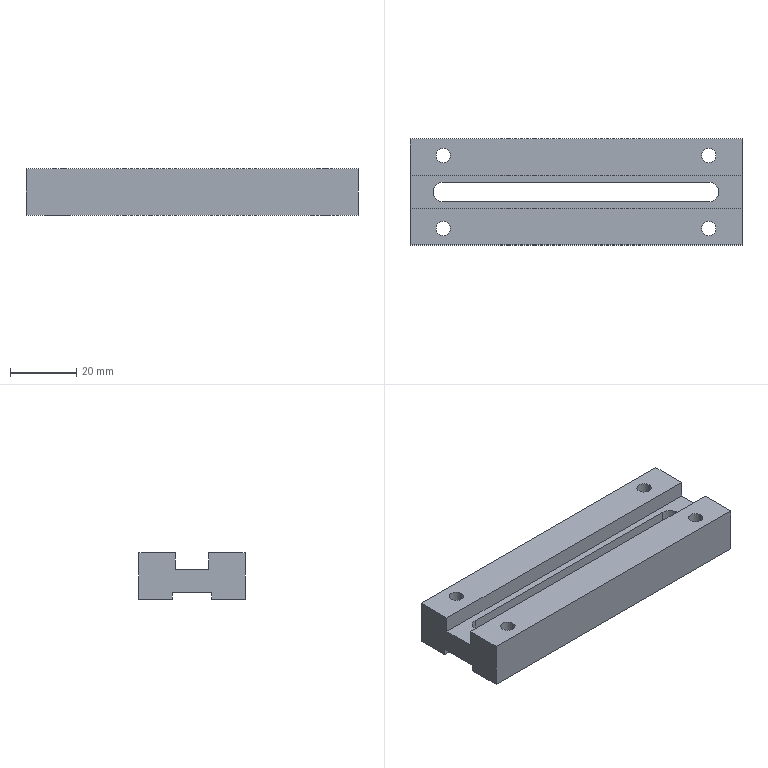Part | NX | features BREP 1 | 1 solid | 39 faces | box 100 x 31.94 x 14 mm | volume 32316 mm3 | plane 20 | cylinder 19 | commonest cylinder face diameters 4.3 x8 8 x8 6 x3
STEP:
#1=CARTESIAN_POINT('',(-36.,-11.,4.4));
#2=VERTEX_POINT('',#1);
#3=CARTESIAN_POINT('',(-44.,-11.,4.4));
#4=VERTEX_POINT('',#3);
#5=CARTESIAN_POINT('',(-40.,-11.,4.4));
#6=DIRECTION('',(0.,0.,-1.));
#7=DIRECTION('',(-1.,0.,0.));
#8=AXIS2_PLACEMENT_3D('',#5,#6,#7);
#9=CIRCLE('',#8,4.);
#10=EDGE_CURVE('',#2,#4,#9,.T.);
#11=ORIENTED_EDGE('',*,*,#10,.F.);
#12=CARTESIAN_POINT('',(-36.,-11.,0.));
#13=VERTEX_POINT('',#12);
#14=CARTESIAN_POINT('',(-36.,-11.,0.));
#15=DIRECTION('',(0.,0.,-1.));
#16=VECTOR('',#15,1000.);
#17=LINE('',#14,#16);
#18=EDGE_CURVE('',#2,#13,#17,.T.);
#19=ORIENTED_EDGE('',*,*,#18,.T.);
#20=CARTESIAN_POINT('',(-44.,-11.,0.));
#21=VERTEX_POINT('',#20);
#22=CARTESIAN_POINT('',(-40.,-11.,0.));
#23=DIRECTION('',(0.,0.,-1.));
#24=DIRECTION('',(-1.,0.,0.));
#25=AXIS2_PLACEMENT_3D('',#22,#23,#24);
#26=CIRCLE('',#25,4.);
#27=EDGE_CURVE('',#13,#21,#26,.T.);
#28=ORIENTED_EDGE('',*,*,#27,.T.);
#29=CARTESIAN_POINT('',(-44.,-11.,0.));
#30=DIRECTION('',(0.,0.,-1.));
#31=VECTOR('',#30,1000.);
#32=LINE('',#29,#31);
#33=EDGE_CURVE('',#4,#21,#32,.T.);
#34=ORIENTED_EDGE('',*,*,#33,.F.);
#35=EDGE_LOOP('',(#11,#19,#28,#34));
#36=FACE_BOUND('',#35,.T.);
#37=CARTESIAN_POINT('',(-40.,-11.,0.));
#38=DIRECTION('',(0.,0.,-1.));
#39=DIRECTION('',(-1.,0.,0.));
#40=AXIS2_PLACEMENT_3D('',#37,#38,#39);
#41=CYLINDRICAL_SURFACE('',#40,4.);
#42=ADVANCED_FACE('',(#36),#41,.F.);
#43=CARTESIAN_POINT('',(-37.85,-11.,14.));
#44=VERTEX_POINT('',#43);
#45=CARTESIAN_POINT('',(-42.15,-11.,14.));
#46=VERTEX_POINT('',#45);
#47=CARTESIAN_POINT('',(-40.,-11.,14.));
#48=DIRECTION('',(0.,0.,-1.));
#49=DIRECTION('',(-1.,0.,0.));
#50=AXIS2_PLACEMENT_3D('',#47,#48,#49);
#51=CIRCLE('',#50,2.15);
#52=EDGE_CURVE('',#44,#46,#51,.T.);
#53=ORIENTED_EDGE('',*,*,#52,.F.);
#54=CARTESIAN_POINT('',(-37.85,-11.,4.4));
#55=VERTEX_POINT('',#54);
#56=CARTESIAN_POINT('',(-37.85,-11.,0.));
#57=DIRECTION('',(0.,0.,-1.));
#58=VECTOR('',#57,1000.);
#59=LINE('',#56,#58);
#60=EDGE_CURVE('',#44,#55,#59,.T.);
#61=ORIENTED_EDGE('',*,*,#60,.T.);
#62=CARTESIAN_POINT('',(-42.15,-11.,4.4));
#63=VERTEX_POINT('',#62);
#64=CARTESIAN_POINT('',(-40.,-11.,4.4));
#65=DIRECTION('',(0.,0.,-1.));
#66=DIRECTION('',(-1.,0.,0.));
#67=AXIS2_PLACEMENT_3D('',#64,#65,#66);
#68=CIRCLE('',#67,2.15);
#69=EDGE_CURVE('',#55,#63,#68,.T.);
#70=ORIENTED_EDGE('',*,*,#69,.T.);
#71=CARTESIAN_POINT('',(-42.15,-11.,0.));
#72=DIRECTION('',(0.,0.,-1.));
#73=VECTOR('',#72,1000.);
#74=LINE('',#71,#73);
#75=EDGE_CURVE('',#46,#63,#74,.T.);
#76=ORIENTED_EDGE('',*,*,#75,.F.);
#77=EDGE_LOOP('',(#53,#61,#70,#76));
#78=FACE_BOUND('',#77,.T.);
#79=CARTESIAN_POINT('',(-40.,-11.,0.));
#80=DIRECTION('',(0.,0.,-1.));
#81=DIRECTION('',(-1.,0.,0.));
#82=AXIS2_PLACEMENT_3D('',#79,#80,#81);
#83=CYLINDRICAL_SURFACE('',#82,2.15);
#84=ADVANCED_FACE('',(#78),#83,.F.);
#85=CARTESIAN_POINT('',(44.,-11.,4.4));
#86=VERTEX_POINT('',#85);
#87=CARTESIAN_POINT('',(36.,-11.,4.4));
#88=VERTEX_POINT('',#87);
#89=CARTESIAN_POINT('',(40.,-11.,4.4));
#90=DIRECTION('',(0.,0.,-1.));
#91=DIRECTION('',(-1.,0.,0.));
#92=AXIS2_PLACEMENT_3D('',#89,#90,#91);
#93=CIRCLE('',#92,4.);
#94=EDGE_CURVE('',#86,#88,#93,.T.);
#95=ORIENTED_EDGE('',*,*,#94,.F.);
#96=CARTESIAN_POINT('',(44.,-11.,0.));
#97=VERTEX_POINT('',#96);
#98=CARTESIAN_POINT('',(44.,-11.,0.));
#99=DIRECTION('',(0.,0.,-1.));
#100=VECTOR('',#99,1000.);
#101=LINE('',#98,#100);
#102=EDGE_CURVE('',#86,#97,#101,.T.);
#103=ORIENTED_EDGE('',*,*,#102,.T.);
#104=CARTESIAN_POINT('',(36.,-11.,0.));
#105=VERTEX_POINT('',#104);
#106=CARTESIAN_POINT('',(40.,-11.,0.));
#107=DIRECTION('',(0.,0.,-1.));
#108=DIRECTION('',(-1.,0.,0.));
#109=AXIS2_PLACEMENT_3D('',#106,#107,#108);
#110=CIRCLE('',#109,4.);
#111=EDGE_CURVE('',#97,#105,#110,.T.);
#112=ORIENTED_EDGE('',*,*,#111,.T.);
#113=CARTESIAN_POINT('',(36.,-11.,0.));
#114=DIRECTION('',(0.,0.,-1.));
#115=VECTOR('',#114,1000.);
#116=LINE('',#113,#115);
#117=EDGE_CURVE('',#88,#105,#116,.T.);
#118=ORIENTED_EDGE('',*,*,#117,.F.);
#119=EDGE_LOOP('',(#95,#103,#112,#118));
#120=FACE_BOUND('',#119,.T.);
#121=CARTESIAN_POINT('',(40.,-11.,0.));
#122=DIRECTION('',(0.,0.,-1.));
#123=DIRECTION('',(-1.,0.,0.));
#124=AXIS2_PLACEMENT_3D('',#121,#122,#123);
#125=CYLINDRICAL_SURFACE('',#124,4.);
#126=ADVANCED_FACE('',(#120),#125,.F.);
#127=CARTESIAN_POINT('',(42.15,-11.,14.));
#128=VERTEX_POINT('',#127);
#129=CARTESIAN_POINT('',(37.85,-11.,14.));
#130=VERTEX_POINT('',#129);
#131=CARTESIAN_POINT('',(40.,-11.,14.));
#132=DIRECTION('',(0.,0.,-1.));
#133=DIRECTION('',(-1.,0.,0.));
#134=AXIS2_PLACEMENT_3D('',#131,#132,#133);
#135=CIRCLE('',#134,2.15);
#136=EDGE_CURVE('',#128,#130,#135,.T.);
#137=ORIENTED_EDGE('',*,*,#136,.F.);
#138=CARTESIAN_POINT('',(42.15,-11.,4.4));
#139=VERTEX_POINT('',#138);
#140=CARTESIAN_POINT('',(42.15,-11.,0.));
#141=DIRECTION('',(0.,0.,-1.));
#142=VECTOR('',#141,1000.);
#143=LINE('',#140,#142);
#144=EDGE_CURVE('',#128,#139,#143,.T.);
#145=ORIENTED_EDGE('',*,*,#144,.T.);
#146=CARTESIAN_POINT('',(37.85,-11.,4.4));
#147=VERTEX_POINT('',#146);
#148=CARTESIAN_POINT('',(40.,-11.,4.4));
#149=DIRECTION('',(0.,0.,-1.));
#150=DIRECTION('',(-1.,0.,0.));
#151=AXIS2_PLACEMENT_3D('',#148,#149,#150);
#152=CIRCLE('',#151,2.15);
#153=EDGE_CURVE('',#139,#147,#152,.T.);
#154=ORIENTED_EDGE('',*,*,#153,.T.);
#155=CARTESIAN_POINT('',(37.85,-11.,0.));
#156=DIRECTION('',(0.,0.,-1.));
#157=VECTOR('',#156,1000.);
#158=LINE('',#155,#157);
#159=EDGE_CURVE('',#130,#147,#158,.T.);
#160=ORIENTED_EDGE('',*,*,#159,.F.);
#161=EDGE_LOOP('',(#137,#145,#154,#160));
#162=FACE_BOUND('',#161,.T.);
#163=CARTESIAN_POINT('',(40.,-11.,0.));
#164=DIRECTION('',(0.,0.,-1.));
#165=DIRECTION('',(-1.,0.,0.));
#166=AXIS2_PLACEMENT_3D('',#163,#164,#165);
#167=CYLINDRICAL_SURFACE('',#166,2.15);
#168=ADVANCED_FACE('',(#162),#167,.F.);
#169=CARTESIAN_POINT('',(-36.,11.,4.4));
#170=VERTEX_POINT('',#169);
#171=CARTESIAN_POINT('',(-44.,11.,4.4));
#172=VERTEX_POINT('',#171);
#173=CARTESIAN_POINT('',(-40.,11.,4.4));
#174=DIRECTION('',(0.,0.,-1.));
#175=DIRECTION('',(-1.,0.,0.));
#176=AXIS2_PLACEMENT_3D('',#173,#174,#175);
#177=CIRCLE('',#176,4.);
#178=EDGE_CURVE('',#170,#172,#177,.T.);
#179=ORIENTED_EDGE('',*,*,#178,.F.);
#180=CARTESIAN_POINT('',(-36.,11.,0.));
#181=VERTEX_POINT('',#180);
#182=CARTESIAN_POINT('',(-36.,11.,0.));
#183=DIRECTION('',(0.,0.,-1.));
#184=VECTOR('',#183,1000.);
#185=LINE('',#182,#184);
#186=EDGE_CURVE('',#170,#181,#185,.T.);
#187=ORIENTED_EDGE('',*,*,#186,.T.);
#188=CARTESIAN_POINT('',(-44.,11.,0.));
#189=VERTEX_POINT('',#188);
#190=CARTESIAN_POINT('',(-40.,11.,0.));
#191=DIRECTION('',(0.,0.,-1.));
#192=DIRECTION('',(-1.,0.,0.));
#193=AXIS2_PLACEMENT_3D('',#190,#191,#192);
#194=CIRCLE('',#193,4.);
#195=EDGE_CURVE('',#181,#189,#194,.T.);
#196=ORIENTED_EDGE('',*,*,#195,.T.);
#197=CARTESIAN_POINT('',(-44.,11.,0.));
#198=DIRECTION('',(0.,0.,-1.));
#199=VECTOR('',#198,1000.);
#200=LINE('',#197,#199);
#201=EDGE_CURVE('',#172,#189,#200,.T.);
#202=ORIENTED_EDGE('',*,*,#201,.F.);
#203=EDGE_LOOP('',(#179,#187,#196,#202));
#204=FACE_BOUND('',#203,.T.);
#205=CARTESIAN_POINT('',(-40.,11.,0.));
#206=DIRECTION('',(0.,0.,-1.));
#207=DIRECTION('',(-1.,0.,0.));
#208=AXIS2_PLACEMENT_3D('',#205,#206,#207);
#209=CYLINDRICAL_SURFACE('',#208,4.);
#210=ADVANCED_FACE('',(#204),#209,.F.);
#211=CARTESIAN_POINT('',(-37.85,11.,14.));
#212=VERTEX_POINT('',#211);
#213=CARTESIAN_POINT('',(-42.15,11.,14.));
#214=VERTEX_POINT('',#213);
#215=CARTESIAN_POINT('',(-40.,11.,14.));
#216=DIRECTION('',(0.,0.,-1.));
#217=DIRECTION('',(-1.,0.,0.));
#218=AXIS2_PLACEMENT_3D('',#215,#216,#217);
#219=CIRCLE('',#218,2.15);
#220=EDGE_CURVE('',#212,#214,#219,.T.);
#221=ORIENTED_EDGE('',*,*,#220,.F.);
#222=CARTESIAN_POINT('',(-37.85,11.,4.4));
#223=VERTEX_POINT('',#222);
#224=CARTESIAN_POINT('',(-37.85,11.,0.));
#225=DIRECTION('',(0.,0.,-1.));
#226=VECTOR('',#225,1000.);
#227=LINE('',#224,#226);
#228=EDGE_CURVE('',#212,#223,#227,.T.);
#229=ORIENTED_EDGE('',*,*,#228,.T.);
#230=CARTESIAN_POINT('',(-42.15,11.,4.4));
#231=VERTEX_POINT('',#230);
#232=CARTESIAN_POINT('',(-40.,11.,4.4));
#233=DIRECTION('',(0.,0.,-1.));
#234=DIRECTION('',(-1.,0.,0.));
#235=AXIS2_PLACEMENT_3D('',#232,#233,#234);
#236=CIRCLE('',#235,2.15);
#237=EDGE_CURVE('',#223,#231,#236,.T.);
#238=ORIENTED_EDGE('',*,*,#237,.T.);
#239=CARTESIAN_POINT('',(-42.15,11.,0.));
#240=DIRECTION('',(0.,0.,-1.));
#241=VECTOR('',#240,1000.);
#242=LINE('',#239,#241);
#243=EDGE_CURVE('',#214,#231,#242,.T.);
#244=ORIENTED_EDGE('',*,*,#243,.F.);
#245=EDGE_LOOP('',(#221,#229,#238,#244));
#246=FACE_BOUND('',#245,.T.);
#247=CARTESIAN_POINT('',(-40.,11.,0.));
#248=DIRECTION('',(0.,0.,-1.));
#249=DIRECTION('',(-1.,0.,0.));
#250=AXIS2_PLACEMENT_3D('',#247,#248,#249);
#251=CYLINDRICAL_SURFACE('',#250,2.15);
#252=ADVANCED_FACE('',(#246),#251,.F.);
#253=CARTESIAN_POINT('',(44.,11.,4.4));
#254=VERTEX_POINT('',#253);
#255=CARTESIAN_POINT('',(36.,11.,4.4));
#256=VERTEX_POINT('',#255);
#257=CARTESIAN_POINT('',(40.,11.,4.4));
#258=DIRECTION('',(0.,0.,-1.));
#259=DIRECTION('',(-1.,0.,0.));
#260=AXIS2_PLACEMENT_3D('',#257,#258,#259);
#261=CIRCLE('',#260,4.);
#262=EDGE_CURVE('',#254,#256,#261,.T.);
#263=ORIENTED_EDGE('',*,*,#262,.F.);
#264=CARTESIAN_POINT('',(44.,11.,0.));
#265=VERTEX_POINT('',#264);
#266=CARTESIAN_POINT('',(44.,11.,0.));
#267=DIRECTION('',(0.,0.,-1.));
#268=VECTOR('',#267,1000.);
#269=LINE('',#266,#268);
#270=EDGE_CURVE('',#254,#265,#269,.T.);
#271=ORIENTED_EDGE('',*,*,#270,.T.);
#272=CARTESIAN_POINT('',(36.,11.,0.));
#273=VERTEX_POINT('',#272);
#274=CARTESIAN_POINT('',(40.,11.,0.));
#275=DIRECTION('',(0.,0.,-1.));
#276=DIRECTION('',(-1.,0.,0.));
#277=AXIS2_PLACEMENT_3D('',#274,#275,#276);
#278=CIRCLE('',#277,4.);
#279=EDGE_CURVE('',#265,#273,#278,.T.);
#280=ORIENTED_EDGE('',*,*,#279,.T.);
#281=CARTESIAN_POINT('',(36.,11.,0.));
#282=DIRECTION('',(0.,0.,-1.));
#283=VECTOR('',#282,1000.);
#284=LINE('',#281,#283);
#285=EDGE_CURVE('',#256,#273,#284,.T.);
#286=ORIENTED_EDGE('',*,*,#285,.F.);
#287=EDGE_LOOP('',(#263,#271,#280,#286));
#288=FACE_BOUND('',#287,.T.);
#289=CARTESIAN_POINT('',(40.,11.,0.));
#290=DIRECTION('',(0.,0.,-1.));
#291=DIRECTION('',(-1.,0.,0.));
#292=AXIS2_PLACEMENT_3D('',#289,#290,#291);
#293=CYLINDRICAL_SURFACE('',#292,4.);
#294=ADVANCED_FACE('',(#288),#293,.F.);
#295=CARTESIAN_POINT('',(42.15,11.,14.));
#296=VERTEX_POINT('',#295);
#297=CARTESIAN_POINT('',(37.85,11.,14.));
#298=VERTEX_POINT('',#297);
#299=CARTESIAN_POINT('',(40.,11.,14.));
#300=DIRECTION('',(0.,0.,-1.));
#301=DIRECTION('',(-1.,0.,0.));
#302=AXIS2_PLACEMENT_3D('',#299,#300,#301);
#303=CIRCLE('',#302,2.15);
#304=EDGE_CURVE('',#296,#298,#303,.T.);
#305=ORIENTED_EDGE('',*,*,#304,.F.);
#306=CARTESIAN_POINT('',(42.15,11.,4.4));
#307=VERTEX_POINT('',#306);
#308=CARTESIAN_POINT('',(42.15,11.,0.));
#309=DIRECTION('',(0.,0.,-1.));
#310=VECTOR('',#309,1000.);
#311=LINE('',#308,#310);
#312=EDGE_CURVE('',#296,#307,#311,.T.);
#313=ORIENTED_EDGE('',*,*,#312,.T.);
#314=CARTESIAN_POINT('',(37.85,11.,4.4));
#315=VERTEX_POINT('',#314);
#316=CARTESIAN_POINT('',(40.,11.,4.4));
#317=DIRECTION('',(0.,0.,-1.));
#318=DIRECTION('',(-1.,0.,0.));
#319=AXIS2_PLACEMENT_3D('',#316,#317,#318);
#320=CIRCLE('',#319,2.15);
#321=EDGE_CURVE('',#307,#315,#320,.T.);
#322=ORIENTED_EDGE('',*,*,#321,.T.);
#323=CARTESIAN_POINT('',(37.85,11.,0.));
#324=DIRECTION('',(0.,0.,-1.));
#325=VECTOR('',#324,1000.);
#326=LINE('',#323,#325);
#327=EDGE_CURVE('',#298,#315,#326,.T.);
#328=ORIENTED_EDGE('',*,*,#327,.F.);
#329=EDGE_LOOP('',(#305,#313,#322,#328));
#330=FACE_BOUND('',#329,.T.);
#331=CARTESIAN_POINT('',(40.,11.,0.));
#332=DIRECTION('',(0.,0.,-1.));
#333=DIRECTION('',(-1.,0.,0.));
#334=AXIS2_PLACEMENT_3D('',#331,#332,#333);
#335=CYLINDRICAL_SURFACE('',#334,2.15);
#336=ADVANCED_FACE('',(#330),#335,.F.);
#337=CARTESIAN_POINT('',(-43.,0.,9.));
#338=VERTEX_POINT('',#337);
#339=CARTESIAN_POINT('',(-40.,3.,9.));
#340=VERTEX_POINT('',#339);
#341=CARTESIAN_POINT('',(-40.,0.,9.));
#342=DIRECTION('',(0.,0.,-1.));
#343=DIRECTION('',(1.,0.,0.));
#344=AXIS2_PLACEMENT_3D('',#341,#342,#343);
#345=CIRCLE('',#344,3.);
#346=EDGE_CURVE('',#338,#340,#345,.T.);
#347=ORIENTED_EDGE('',*,*,#346,.F.);
#348=CARTESIAN_POINT('',(-43.,0.,2.));
#349=VERTEX_POINT('',#348);
#350=CARTESIAN_POINT('',(-43.,0.,14.));
#351=DIRECTION('',(0.,0.,-1.));
#352=VECTOR('',#351,1000.);
#353=LINE('',#350,#352);
#354=EDGE_CURVE('',#338,#349,#353,.T.);
#355=ORIENTED_EDGE('',*,*,#354,.T.);
#356=CARTESIAN_POINT('',(-40.,3.,2.));
#357=VERTEX_POINT('',#356);
#358=CARTESIAN_POINT('',(-40.,0.,2.));
#359=DIRECTION('',(0.,0.,-1.));
#360=DIRECTION('',(-1.,0.,0.));
#361=AXIS2_PLACEMENT_3D('',#358,#359,#360);
#362=CIRCLE('',#361,3.);
#363=EDGE_CURVE('',#349,#357,#362,.T.);
#364=ORIENTED_EDGE('',*,*,#363,.T.);
#365=CARTESIAN_POINT('',(-40.,3.,14.));
#366=DIRECTION('',(0.,0.,-1.));
#367=VECTOR('',#366,1000.);
#368=LINE('',#365,#367);
#369=EDGE_CURVE('',#340,#357,#368,.T.);
#370=ORIENTED_EDGE('',*,*,#369,.F.);
#371=EDGE_LOOP('',(#347,#355,#364,#370));
#372=FACE_BOUND('',#371,.T.);
#373=CARTESIAN_POINT('',(-40.,0.,14.));
#374=DIRECTION('',(0.,0.,-1.));
#375=DIRECTION('',(-1.,0.,0.));
#376=AXIS2_PLACEMENT_3D('',#373,#374,#375);
#377=CYLINDRICAL_SURFACE('',#376,3.);
#378=ADVANCED_FACE('',(#372),#377,.F.);
#379=CARTESIAN_POINT('',(50.,-15.97,14.));
#380=VERTEX_POINT('',#379);
#381=CARTESIAN_POINT('',(50.,-5.,14.));
#382=VERTEX_POINT('',#381);
#383=CARTESIAN_POINT('',(50.,-16.,14.));
#384=DIRECTION('',(0.,1.,0.));
#385=VECTOR('',#384,1000.);
#386=LINE('',#383,#385);
#387=EDGE_CURVE('',#380,#382,#386,.T.);
#388=ORIENTED_EDGE('',*,*,#387,.T.);
#389=CARTESIAN_POINT('',(-50.,-5.,14.));
#390=VERTEX_POINT('',#389);
#391=CARTESIAN_POINT('',(-53.992,-5.,14.));
#392=DIRECTION('',(1.,0.,0.));
#393=VECTOR('',#392,1000.);
#394=LINE('',#391,#393);
#395=EDGE_CURVE('',#390,#382,#394,.T.);
#396=ORIENTED_EDGE('',*,*,#395,.F.);
#397=CARTESIAN_POINT('',(-50.,-15.97,14.));
#398=VERTEX_POINT('',#397);
#399=CARTESIAN_POINT('',(-50.,-16.,14.));
#400=DIRECTION('',(0.,-1.,0.));
#401=VECTOR('',#400,1000.);
#402=LINE('',#399,#401);
#403=EDGE_CURVE('',#390,#398,#402,.T.);
#404=ORIENTED_EDGE('',*,*,#403,.T.);
#405=CARTESIAN_POINT('',(-50.,-15.97,14.));
#406=DIRECTION('',(1.,0.,0.));
#407=VECTOR('',#406,1000.);
#408=LINE('',#405,#407);
#409=EDGE_CURVE('',#398,#380,#408,.T.);
#410=ORIENTED_EDGE('',*,*,#409,.T.);
#411=EDGE_LOOP('',(#388,#396,#404,#410));
#412=FACE_BOUND('',#411,.T.);
#413=CARTESIAN_POINT('',(-40.,-11.,14.));
#414=DIRECTION('',(0.,0.,-1.));
#415=DIRECTION('',(-1.,0.,0.));
#416=AXIS2_PLACEMENT_3D('',#413,#414,#415);
#417=CIRCLE('',#416,2.15);
#418=EDGE_CURVE('',#46,#44,#417,.T.);
#419=ORIENTED_EDGE('',*,*,#418,.T.);
#420=ORIENTED_EDGE('',*,*,#52,.T.);
#421=EDGE_LOOP('',(#419,#420));
#422=FACE_BOUND('',#421,.T.);
#423=CARTESIAN_POINT('',(40.,-11.,14.));
#424=DIRECTION('',(0.,0.,-1.));
#425=DIRECTION('',(-1.,0.,0.));
#426=AXIS2_PLACEMENT_3D('',#423,#424,#425);
#427=CIRCLE('',#426,2.15);
#428=EDGE_CURVE('',#130,#128,#427,.T.);
#429=ORIENTED_EDGE('',*,*,#428,.T.);
#430=ORIENTED_EDGE('',*,*,#136,.T.);
#431=EDGE_LOOP('',(#429,#430));
#432=FACE_BOUND('',#431,.T.);
#433=CARTESIAN_POINT('',(0.,0.,14.));
#434=DIRECTION('',(0.,0.,-1.));
#435=DIRECTION('',(0.,-1.,0.));
#436=AXIS2_PLACEMENT_3D('',#433,#434,#435);
#437=PLANE('',#436);
#438=ADVANCED_FACE('',(#412,#422,#432),#437,.F.);
#439=CARTESIAN_POINT('',(40.,3.,9.));
#440=VERTEX_POINT('',#439);
#441=CARTESIAN_POINT('',(40.,-3.,9.));
#442=VERTEX_POINT('',#441);
#443=CARTESIAN_POINT('',(40.,0.,9.));
#444=DIRECTION('',(0.,0.,-1.));
#445=DIRECTION('',(1.,0.,0.));
#446=AXIS2_PLACEMENT_3D('',#443,#444,#445);
#447=CIRCLE('',#446,3.);
#448=EDGE_CURVE('',#440,#442,#447,.T.);
#449=ORIENTED_EDGE('',*,*,#448,.F.);
#450=CARTESIAN_POINT('',(40.,3.,2.));
#451=VERTEX_POINT('',#450);
#452=CARTESIAN_POINT('',(40.,3.,14.));
#453=DIRECTION('',(0.,0.,-1.));
#454=VECTOR('',#453,1000.);
#455=LINE('',#452,#454);
#456=EDGE_CURVE('',#440,#451,#455,.T.);
#457=ORIENTED_EDGE('',*,*,#456,.T.);
#458=CARTESIAN_POINT('',(40.,-3.,2.));
#459=VERTEX_POINT('',#458);
#460=CARTESIAN_POINT('',(40.,0.,2.));
#461=DIRECTION('',(0.,0.,-1.));
#462=DIRECTION('',(-1.,0.,0.));
#463=AXIS2_PLACEMENT_3D('',#460,#461,#462);
#464=CIRCLE('',#463,3.);
#465=EDGE_CURVE('',#451,#459,#464,.T.);
#466=ORIENTED_EDGE('',*,*,#465,.T.);
#467=CARTESIAN_POINT('',(40.,-3.,14.));
#468=DIRECTION('',(0.,0.,-1.));
#469=VECTOR('',#468,1000.);
#470=LINE('',#467,#469);
#471=EDGE_CURVE('',#442,#459,#470,.T.);
#472=ORIENTED_EDGE('',*,*,#471,.F.);
#473=EDGE_LOOP('',(#449,#457,#466,#472));
#474=FACE_BOUND('',#473,.T.);
#475=CARTESIAN_POINT('',(40.,0.,14.));
#476=DIRECTION('',(0.,0.,-1.));
#477=DIRECTION('',(-1.,0.,0.));
#478=AXIS2_PLACEMENT_3D('',#475,#476,#477);
#479=CYLINDRICAL_SURFACE('',#478,3.);
#480=ADVANCED_FACE('',(#474),#479,.F.);
#481=CARTESIAN_POINT('',(40.,3.,9.));
#482=DIRECTION('',(1.,0.,0.));
#483=VECTOR('',#482,1000.);
#484=LINE('',#481,#483);
#485=EDGE_CURVE('',#340,#440,#484,.T.);
#486=ORIENTED_EDGE('',*,*,#485,.F.);
#487=ORIENTED_EDGE('',*,*,#369,.T.);
#488=CARTESIAN_POINT('',(40.,3.,2.));
#489=DIRECTION('',(1.,0.,0.));
#490=VECTOR('',#489,1000.);
#491=LINE('',#488,#490);
#492=EDGE_CURVE('',#357,#451,#491,.T.);
#493=ORIENTED_EDGE('',*,*,#492,.T.);
#494=ORIENTED_EDGE('',*,*,#456,.F.);
#495=EDGE_LOOP('',(#486,#487,#493,#494));
#496=FACE_BOUND('',#495,.T.);
#497=CARTESIAN_POINT('',(40.,3.,14.));
#498=DIRECTION('',(0.,1.,0.));
#499=DIRECTION('',(1.,0.,0.));
#500=AXIS2_PLACEMENT_3D('',#497,#498,#499);
#501=PLANE('',#500);
#502=ADVANCED_FACE('',(#496),#501,.F.);
#503=ORIENTED_EDGE('',*,*,#354,.F.);
#504=CARTESIAN_POINT('',(-40.,-3.,9.));
#505=VERTEX_POINT('',#504);
#506=CARTESIAN_POINT('',(-40.,0.,9.));
#507=DIRECTION('',(0.,0.,-1.));
#508=DIRECTION('',(1.,0.,0.));
#509=AXIS2_PLACEMENT_3D('',#506,#507,#508);
#510=CIRCLE('',#509,3.);
#511=EDGE_CURVE('',#505,#338,#510,.T.);
#512=ORIENTED_EDGE('',*,*,#511,.F.);
#513=CARTESIAN_POINT('',(-40.,-3.,2.));
#514=VERTEX_POINT('',#513);
#515=CARTESIAN_POINT('',(-40.,-3.,14.));
#516=DIRECTION('',(0.,0.,-1.));
#517=VECTOR('',#516,1000.);
#518=LINE('',#515,#517);
#519=EDGE_CURVE('',#505,#514,#518,.T.);
#520=ORIENTED_EDGE('',*,*,#519,.T.);
#521=CARTESIAN_POINT('',(-40.,0.,2.));
#522=DIRECTION('',(0.,0.,-1.));
#523=DIRECTION('',(-1.,0.,0.));
#524=AXIS2_PLACEMENT_3D('',#521,#522,#523);
#525=CIRCLE('',#524,3.);
#526=EDGE_CURVE('',#514,#349,#525,.T.);
#527=ORIENTED_EDGE('',*,*,#526,.T.);
#528=EDGE_LOOP('',(#503,#512,#520,#527));
#529=FACE_BOUND('',#528,.T.);
#530=CARTESIAN_POINT('',(-40.,0.,14.));
#531=DIRECTION('',(0.,0.,-1.));
#532=DIRECTION('',(-1.,0.,0.));
#533=AXIS2_PLACEMENT_3D('',#530,#531,#532);
#534=CYLINDRICAL_SURFACE('',#533,3.);
#535=ADVANCED_FACE('',(#529),#534,.F.);
#536=CARTESIAN_POINT('',(40.,-3.,9.));
#537=DIRECTION('',(-1.,0.,0.));
#538=VECTOR('',#537,1000.);
#539=LINE('',#536,#538);
#540=EDGE_CURVE('',#442,#505,#539,.T.);
#541=ORIENTED_EDGE('',*,*,#540,.F.);
#542=ORIENTED_EDGE('',*,*,#471,.T.);
#543=CARTESIAN_POINT('',(40.,-3.,2.));
#544=DIRECTION('',(-1.,0.,0.));
#545=VECTOR('',#544,1000.);
#546=LINE('',#543,#545);
#547=EDGE_CURVE('',#459,#514,#546,.T.);
#548=ORIENTED_EDGE('',*,*,#547,.T.);
#549=ORIENTED_EDGE('',*,*,#519,.F.);
#550=EDGE_LOOP('',(#541,#542,#548,#549));
#551=FACE_BOUND('',#550,.T.);
#552=CARTESIAN_POINT('',(40.,-3.,14.));
#553=DIRECTION('',(0.,-1.,0.));
#554=DIRECTION('',(-1.,0.,0.));
#555=AXIS2_PLACEMENT_3D('',#552,#553,#554);
#556=PLANE('',#555);
#557=ADVANCED_FACE('',(#551),#556,.F.);
#558=CARTESIAN_POINT('',(-50.,6.,0.));
#559=VERTEX_POINT('',#558);
#560=CARTESIAN_POINT('',(50.,6.,0.));
#561=VERTEX_POINT('',#560);
#562=CARTESIAN_POINT('',(0.,6.,0.));
#563=DIRECTION('',(1.,0.,0.));
#564=VECTOR('',#563,1000.);
#565=LINE('',#562,#564);
#566=EDGE_CURVE('',#559,#561,#565,.T.);
#567=ORIENTED_EDGE('',*,*,#566,.F.);
#568=CARTESIAN_POINT('',(-50.,15.97,0.));
#569=VERTEX_POINT('',#568);
#570=CARTESIAN_POINT('',(-50.,-16.,0.));
#571=DIRECTION('',(0.,-1.,0.));
#572=VECTOR('',#571,1000.);
#573=LINE('',#570,#572);
#574=EDGE_CURVE('',#569,#559,#573,.T.);
#575=ORIENTED_EDGE('',*,*,#574,.F.);
#576=CARTESIAN_POINT('',(50.,15.97,0.));
#577=VERTEX_POINT('',#576);
#578=CARTESIAN_POINT('',(-50.,15.97,0.));
#579=DIRECTION('',(-1.,0.,0.));
#580=VECTOR('',#579,1000.);
#581=LINE('',#578,#580);
#582=EDGE_CURVE('',#577,#569,#581,.T.);
#583=ORIENTED_EDGE('',*,*,#582,.F.);
#584=CARTESIAN_POINT('',(50.,-16.,0.));
#585=DIRECTION('',(0.,1.,0.));
#586=VECTOR('',#585,1000.);
#587=LINE('',#584,#586);
#588=EDGE_CURVE('',#561,#577,#587,.T.);
#589=ORIENTED_EDGE('',*,*,#588,.F.);
#590=EDGE_LOOP('',(#567,#575,#583,#589));
#591=FACE_BOUND('',#590,.T.);
#592=CARTESIAN_POINT('',(-40.,11.,0.));
#593=DIRECTION('',(0.,0.,-1.));
#594=DIRECTION('',(-1.,0.,0.));
#595=AXIS2_PLACEMENT_3D('',#592,#593,#594);
#596=CIRCLE('',#595,4.);
#597=EDGE_CURVE('',#189,#181,#596,.T.);
#598=ORIENTED_EDGE('',*,*,#597,.F.);
#599=ORIENTED_EDGE('',*,*,#195,.F.);
#600=EDGE_LOOP('',(#598,#599));
#601=FACE_BOUND('',#600,.T.);
#602=CARTESIAN_POINT('',(40.,11.,0.));
#603=DIRECTION('',(0.,0.,-1.));
#604=DIRECTION('',(-1.,0.,0.));
#605=AXIS2_PLACEMENT_3D('',#602,#603,#604);
#606=CIRCLE('',#605,4.);
#607=EDGE_CURVE('',#273,#265,#606,.T.);
#608=ORIENTED_EDGE('',*,*,#607,.F.);
#609=ORIENTED_EDGE('',*,*,#279,.F.);
#610=EDGE_LOOP('',(#608,#609));
#611=FACE_BOUND('',#610,.T.);
#612=CARTESIAN_POINT('',(0.,0.,0.));
#613=DIRECTION('',(0.,0.,-1.));
#614=DIRECTION('',(0.,-1.,0.));
#615=AXIS2_PLACEMENT_3D('',#612,#613,#614);
#616=PLANE('',#615);
#617=ADVANCED_FACE('',(#591,#601,#611),#616,.T.);
#618=CARTESIAN_POINT('',(50.,-5.,9.));
#619=VERTEX_POINT('',#618);
#620=CARTESIAN_POINT('',(50.,5.,9.));
#621=VERTEX_POINT('',#620);
#622=CARTESIAN_POINT('',(50.,-16.,9.));
#623=DIRECTION('',(0.,1.,0.));
#624=VECTOR('',#623,1000.);
#625=LINE('',#622,#624);
#626=EDGE_CURVE('',#619,#621,#625,.T.);
#627=ORIENTED_EDGE('',*,*,#626,.F.);
#628=CARTESIAN_POINT('',(50.,-5.,14.));
#629=DIRECTION('',(0.,0.,1.));
#630=VECTOR('',#629,1000.);
#631=LINE('',#628,#630);
#632=EDGE_CURVE('',#619,#382,#631,.T.);
#633=ORIENTED_EDGE('',*,*,#632,.T.);
#634=ORIENTED_EDGE('',*,*,#387,.F.);
#635=CARTESIAN_POINT('',(50.,-15.97,0.));
#636=VERTEX_POINT('',#635);
#637=CARTESIAN_POINT('',(50.,-15.97,14.));
#638=DIRECTION('',(0.,0.,-1.));
#639=VECTOR('',#638,1000.);
#640=LINE('',#637,#639);
#641=EDGE_CURVE('',#380,#636,#640,.T.);
#642=ORIENTED_EDGE('',*,*,#641,.T.);
#643=CARTESIAN_POINT('',(50.,-6.,0.));
#644=VERTEX_POINT('',#643);
#645=CARTESIAN_POINT('',(50.,-16.,0.));
#646=DIRECTION('',(0.,1.,0.));
#647=VECTOR('',#646,1000.);
#648=LINE('',#645,#647);
#649=EDGE_CURVE('',#636,#644,#648,.T.);
#650=ORIENTED_EDGE('',*,*,#649,.T.);
#651=CARTESIAN_POINT('',(50.,-6.,2.));
#652=VERTEX_POINT('',#651);
#653=CARTESIAN_POINT('',(50.,-6.,14.));
#654=DIRECTION('',(0.,0.,1.));
#655=VECTOR('',#654,1000.);
#656=LINE('',#653,#655);
#657=EDGE_CURVE('',#644,#652,#656,.T.);
#658=ORIENTED_EDGE('',*,*,#657,.T.);
#659=CARTESIAN_POINT('',(50.,6.,2.));
#660=VERTEX_POINT('',#659);
#661=CARTESIAN_POINT('',(50.,-16.,2.));
#662=DIRECTION('',(0.,-1.,0.));
#663=VECTOR('',#662,1000.);
#664=LINE('',#661,#663);
#665=EDGE_CURVE('',#660,#652,#664,.T.);
#666=ORIENTED_EDGE('',*,*,#665,.F.);
#667=CARTESIAN_POINT('',(50.,6.,14.));
#668=DIRECTION('',(0.,0.,-1.));
#669=VECTOR('',#668,1000.);
#670=LINE('',#667,#669);
#671=EDGE_CURVE('',#660,#561,#670,.T.);
#672=ORIENTED_EDGE('',*,*,#671,.T.);
#673=ORIENTED_EDGE('',*,*,#588,.T.);
#674=CARTESIAN_POINT('',(50.,15.97,14.));
#675=VERTEX_POINT('',#674);
#676=CARTESIAN_POINT('',(50.,15.97,14.));
#677=DIRECTION('',(0.,0.,-1.));
#678=VECTOR('',#677,1000.);
#679=LINE('',#676,#678);
#680=EDGE_CURVE('',#675,#577,#679,.T.);
#681=ORIENTED_EDGE('',*,*,#680,.F.);
#682=CARTESIAN_POINT('',(50.,5.,14.));
#683=VERTEX_POINT('',#682);
#684=CARTESIAN_POINT('',(50.,-16.,14.));
#685=DIRECTION('',(0.,1.,0.));
#686=VECTOR('',#685,1000.);
#687=LINE('',#684,#686);
#688=EDGE_CURVE('',#683,#675,#687,.T.);
#689=ORIENTED_EDGE('',*,*,#688,.F.);
#690=CARTESIAN_POINT('',(50.,5.,14.));
#691=DIRECTION('',(0.,0.,-1.));
#692=VECTOR('',#691,1000.);
#693=LINE('',#690,#692);
#694=EDGE_CURVE('',#683,#621,#693,.T.);
#695=ORIENTED_EDGE('',*,*,#694,.T.);
#696=EDGE_LOOP('',(#627,#633,#634,#642,#650,#658,#666,#672,#673,#681,#689,#695));
#697=FACE_BOUND('',#696,.T.);
#698=CARTESIAN_POINT('',(50.,-16.,14.));
#699=DIRECTION('',(-1.,0.,0.));
#700=DIRECTION('',(0.,0.,1.));
#701=AXIS2_PLACEMENT_3D('',#698,#699,#700);
#702=PLANE('',#701);
#703=ADVANCED_FACE('',(#697),#702,.F.);
#704=ORIENTED_EDGE('',*,*,#582,.T.);
#705=CARTESIAN_POINT('',(-50.,15.97,14.));
#706=VERTEX_POINT('',#705);
#707=CARTESIAN_POINT('',(-50.,15.97,14.));
#708=DIRECTION('',(0.,0.,-1.));
#709=VECTOR('',#708,1000.);
#710=LINE('',#707,#709);
#711=EDGE_CURVE('',#706,#569,#710,.T.);
#712=ORIENTED_EDGE('',*,*,#711,.F.);
#713=CARTESIAN_POINT('',(-50.,15.97,14.));
#714=DIRECTION('',(-1.,0.,0.));
#715=VECTOR('',#714,1000.);
#716=LINE('',#713,#715);
#717=EDGE_CURVE('',#675,#706,#716,.T.);
#718=ORIENTED_EDGE('',*,*,#717,.F.);
#719=ORIENTED_EDGE('',*,*,#680,.T.);
#720=EDGE_LOOP('',(#704,#712,#718,#719));
#721=FACE_BOUND('',#720,.T.);
#722=CARTESIAN_POINT('',(-50.,15.97,14.));
#723=DIRECTION('',(0.,-1.,0.));
#724=DIRECTION('',(0.,0.,-1.));
#725=AXIS2_PLACEMENT_3D('',#722,#723,#724);
#726=PLANE('',#725);
#727=ADVANCED_FACE('',(#721),#726,.F.);
#728=ORIENTED_EDGE('',*,*,#403,.F.);
#729=CARTESIAN_POINT('',(-50.,-5.,9.));
#730=VERTEX_POINT('',#729);
#731=CARTESIAN_POINT('',(-50.,-5.,14.));
#732=DIRECTION('',(0.,0.,-1.));
#733=VECTOR('',#732,1000.);
#734=LINE('',#731,#733);
#735=EDGE_CURVE('',#390,#730,#734,.T.);
#736=ORIENTED_EDGE('',*,*,#735,.T.);
#737=CARTESIAN_POINT('',(-50.,5.,9.));
#738=VERTEX_POINT('',#737);
#739=CARTESIAN_POINT('',(-50.,-16.,9.));
#740=DIRECTION('',(0.,-1.,0.));
#741=VECTOR('',#740,1000.);
#742=LINE('',#739,#741);
#743=EDGE_CURVE('',#738,#730,#742,.T.);
#744=ORIENTED_EDGE('',*,*,#743,.F.);
#745=CARTESIAN_POINT('',(-50.,5.,14.));
#746=VERTEX_POINT('',#745);
#747=CARTESIAN_POINT('',(-50.,5.,14.));
#748=DIRECTION('',(0.,0.,1.));
#749=VECTOR('',#748,1000.);
#750=LINE('',#747,#749);
#751=EDGE_CURVE('',#738,#746,#750,.T.);
#752=ORIENTED_EDGE('',*,*,#751,.T.);
#753=CARTESIAN_POINT('',(-50.,-16.,14.));
#754=DIRECTION('',(0.,-1.,0.));
#755=VECTOR('',#754,1000.);
#756=LINE('',#753,#755);
#757=EDGE_CURVE('',#706,#746,#756,.T.);
#758=ORIENTED_EDGE('',*,*,#757,.F.);
#759=ORIENTED_EDGE('',*,*,#711,.T.);
#760=ORIENTED_EDGE('',*,*,#574,.T.);
#761=CARTESIAN_POINT('',(-50.,6.,2.));
#762=VERTEX_POINT('',#761);
#763=CARTESIAN_POINT('',(-50.,6.,14.));
#764=DIRECTION('',(0.,0.,1.));
#765=VECTOR('',#764,1000.);
#766=LINE('',#763,#765);
#767=EDGE_CURVE('',#559,#762,#766,.T.);
#768=ORIENTED_EDGE('',*,*,#767,.T.);
#769=CARTESIAN_POINT('',(-50.,-6.,2.));
#770=VERTEX_POINT('',#769);
#771=CARTESIAN_POINT('',(-50.,-16.,2.));
#772=DIRECTION('',(0.,1.,0.));
#773=VECTOR('',#772,1000.);
#774=LINE('',#771,#773);
#775=EDGE_CURVE('',#770,#762,#774,.T.);
#776=ORIENTED_EDGE('',*,*,#775,.F.);
#777=CARTESIAN_POINT('',(-50.,-6.,0.));
#778=VERTEX_POINT('',#777);
#779=CARTESIAN_POINT('',(-50.,-6.,14.));
#780=DIRECTION('',(0.,0.,-1.));
#781=VECTOR('',#780,1000.);
#782=LINE('',#779,#781);
#783=EDGE_CURVE('',#770,#778,#782,.T.);
#784=ORIENTED_EDGE('',*,*,#783,.T.);
#785=CARTESIAN_POINT('',(-50.,-15.97,0.));
#786=VERTEX_POINT('',#785);
#787=CARTESIAN_POINT('',(-50.,-16.,0.));
#788=DIRECTION('',(0.,-1.,0.));
#789=VECTOR('',#788,1000.);
#790=LINE('',#787,#789);
#791=EDGE_CURVE('',#778,#786,#790,.T.);
#792=ORIENTED_EDGE('',*,*,#791,.T.);
#793=CARTESIAN_POINT('',(-50.,-15.97,14.));
#794=DIRECTION('',(0.,0.,-1.));
#795=VECTOR('',#794,1000.);
#796=LINE('',#793,#795);
#797=EDGE_CURVE('',#398,#786,#796,.T.);
#798=ORIENTED_EDGE('',*,*,#797,.F.);
#799=EDGE_LOOP('',(#728,#736,#744,#752,#758,#759,#760,#768,#776,#784,#792,#798));
#800=FACE_BOUND('',#799,.T.);
#801=CARTESIAN_POINT('',(-50.,-16.,14.));
#802=DIRECTION('',(1.,0.,0.));
#803=DIRECTION('',(0.,1.,0.));
#804=AXIS2_PLACEMENT_3D('',#801,#802,#803);
#805=PLANE('',#804);
#806=ADVANCED_FACE('',(#800),#805,.F.);
#807=CARTESIAN_POINT('',(-50.,-15.97,0.));
#808=DIRECTION('',(1.,0.,0.));
#809=VECTOR('',#808,1000.);
#810=LINE('',#807,#809);
#811=EDGE_CURVE('',#786,#636,#810,.T.);
#812=ORIENTED_EDGE('',*,*,#811,.T.);
#813=ORIENTED_EDGE('',*,*,#641,.F.);
#814=ORIENTED_EDGE('',*,*,#409,.F.);
#815=ORIENTED_EDGE('',*,*,#797,.T.);
#816=EDGE_LOOP('',(#812,#813,#814,#815));
#817=FACE_BOUND('',#816,.T.);
#818=CARTESIAN_POINT('',(-50.,-15.97,14.));
#819=DIRECTION('',(0.,1.,0.));
#820=DIRECTION('',(1.,0.,0.));
#821=AXIS2_PLACEMENT_3D('',#818,#819,#820);
#822=PLANE('',#821);
#823=ADVANCED_FACE('',(#817),#822,.F.);
#824=ORIENTED_EDGE('',*,*,#757,.T.);
#825=CARTESIAN_POINT('',(-53.992,5.,14.));
#826=DIRECTION('',(-1.,0.,0.));
#827=VECTOR('',#826,1000.);
#828=LINE('',#825,#827);
#829=EDGE_CURVE('',#683,#746,#828,.T.);
#830=ORIENTED_EDGE('',*,*,#829,.F.);
#831=ORIENTED_EDGE('',*,*,#688,.T.);
#832=ORIENTED_EDGE('',*,*,#717,.T.);
#833=EDGE_LOOP('',(#824,#830,#831,#832));
#834=FACE_BOUND('',#833,.T.);
#835=CARTESIAN_POINT('',(-40.,11.,14.));
#836=DIRECTION('',(0.,0.,-1.));
#837=DIRECTION('',(-1.,0.,0.));
#838=AXIS2_PLACEMENT_3D('',#835,#836,#837);
#839=CIRCLE('',#838,2.15);
#840=EDGE_CURVE('',#214,#212,#839,.T.);
#841=ORIENTED_EDGE('',*,*,#840,.T.);
#842=ORIENTED_EDGE('',*,*,#220,.T.);
#843=EDGE_LOOP('',(#841,#842));
#844=FACE_BOUND('',#843,.T.);
#845=CARTESIAN_POINT('',(40.,11.,14.));
#846=DIRECTION('',(0.,0.,-1.));
#847=DIRECTION('',(-1.,0.,0.));
#848=AXIS2_PLACEMENT_3D('',#845,#846,#847);
#849=CIRCLE('',#848,2.15);
#850=EDGE_CURVE('',#298,#296,#849,.T.);
#851=ORIENTED_EDGE('',*,*,#850,.T.);
#852=ORIENTED_EDGE('',*,*,#304,.T.);
#853=EDGE_LOOP('',(#851,#852));
#854=FACE_BOUND('',#853,.T.);
#855=CARTESIAN_POINT('',(0.,0.,14.));
#856=DIRECTION('',(0.,0.,-1.));
#857=DIRECTION('',(0.,-1.,0.));
#858=AXIS2_PLACEMENT_3D('',#855,#856,#857);
#859=PLANE('',#858);
#860=ADVANCED_FACE('',(#834,#844,#854),#859,.F.);
#861=CARTESIAN_POINT('',(0.,-6.,0.));
#862=DIRECTION('',(-1.,0.,0.));
#863=VECTOR('',#862,1000.);
#864=LINE('',#861,#863);
#865=EDGE_CURVE('',#644,#778,#864,.T.);
#866=ORIENTED_EDGE('',*,*,#865,.F.);
#867=ORIENTED_EDGE('',*,*,#649,.F.);
#868=ORIENTED_EDGE('',*,*,#811,.F.);
#869=ORIENTED_EDGE('',*,*,#791,.F.);
#870=EDGE_LOOP('',(#866,#867,#868,#869));
#871=FACE_BOUND('',#870,.T.);
#872=CARTESIAN_POINT('',(-40.,-11.,0.));
#873=DIRECTION('',(0.,0.,-1.));
#874=DIRECTION('',(-1.,0.,0.));
#875=AXIS2_PLACEMENT_3D('',#872,#873,#874);
#876=CIRCLE('',#875,4.);
#877=EDGE_CURVE('',#21,#13,#876,.T.);
#878=ORIENTED_EDGE('',*,*,#877,.F.);
#879=ORIENTED_EDGE('',*,*,#27,.F.);
#880=EDGE_LOOP('',(#878,#879));
#881=FACE_BOUND('',#880,.T.);
#882=CARTESIAN_POINT('',(40.,-11.,0.));
#883=DIRECTION('',(0.,0.,-1.));
#884=DIRECTION('',(-1.,0.,0.));
#885=AXIS2_PLACEMENT_3D('',#882,#883,#884);
#886=CIRCLE('',#885,4.);
#887=EDGE_CURVE('',#105,#97,#886,.T.);
#888=ORIENTED_EDGE('',*,*,#887,.F.);
#889=ORIENTED_EDGE('',*,*,#111,.F.);
#890=EDGE_LOOP('',(#888,#889));
#891=FACE_BOUND('',#890,.T.);
#892=CARTESIAN_POINT('',(0.,0.,0.));
#893=DIRECTION('',(0.,0.,-1.));
#894=DIRECTION('',(0.,-1.,0.));
#895=AXIS2_PLACEMENT_3D('',#892,#893,#894);
#896=PLANE('',#895);
#897=ADVANCED_FACE('',(#871,#881,#891),#896,.T.);
#898=ORIENTED_EDGE('',*,*,#665,.T.);
#899=CARTESIAN_POINT('',(-54.873,-6.,2.));
#900=DIRECTION('',(-1.,0.,0.));
#901=VECTOR('',#900,1000.);
#902=LINE('',#899,#901);
#903=EDGE_CURVE('',#652,#770,#902,.T.);
#904=ORIENTED_EDGE('',*,*,#903,.T.);
#905=ORIENTED_EDGE('',*,*,#775,.T.);
#906=CARTESIAN_POINT('',(-54.873,6.,2.));
#907=DIRECTION('',(1.,0.,0.));
#908=VECTOR('',#907,1000.);
#909=LINE('',#906,#908);
#910=EDGE_CURVE('',#762,#660,#909,.T.);
#911=ORIENTED_EDGE('',*,*,#910,.T.);
#912=EDGE_LOOP('',(#898,#904,#905,#911));
#913=FACE_BOUND('',#912,.T.);
#914=ORIENTED_EDGE('',*,*,#465,.F.);
#915=ORIENTED_EDGE('',*,*,#492,.F.);
#916=ORIENTED_EDGE('',*,*,#363,.F.);
#917=ORIENTED_EDGE('',*,*,#526,.F.);
#918=ORIENTED_EDGE('',*,*,#547,.F.);
#919=EDGE_LOOP('',(#914,#915,#916,#917,#918));
#920=FACE_BOUND('',#919,.T.);
#921=CARTESIAN_POINT('',(0.,0.,2.));
#922=DIRECTION('',(0.,0.,-1.));
#923=DIRECTION('',(0.,-1.,0.));
#924=AXIS2_PLACEMENT_3D('',#921,#922,#923);
#925=PLANE('',#924);
#926=ADVANCED_FACE('',(#913,#920),#925,.T.);
#927=ORIENTED_EDGE('',*,*,#910,.F.);
#928=ORIENTED_EDGE('',*,*,#767,.F.);
#929=ORIENTED_EDGE('',*,*,#566,.T.);
#930=ORIENTED_EDGE('',*,*,#671,.F.);
#931=EDGE_LOOP('',(#927,#928,#929,#930));
#932=FACE_BOUND('',#931,.T.);
#933=CARTESIAN_POINT('',(-54.873,6.,2.));
#934=DIRECTION('',(0.,1.,0.));
#935=DIRECTION('',(1.,0.,0.));
#936=AXIS2_PLACEMENT_3D('',#933,#934,#935);
#937=PLANE('',#936);
#938=ADVANCED_FACE('',(#932),#937,.F.);
#939=ORIENTED_EDGE('',*,*,#865,.T.);
#940=ORIENTED_EDGE('',*,*,#783,.F.);
#941=ORIENTED_EDGE('',*,*,#903,.F.);
#942=ORIENTED_EDGE('',*,*,#657,.F.);
#943=EDGE_LOOP('',(#939,#940,#941,#942));
#944=FACE_BOUND('',#943,.T.);
#945=CARTESIAN_POINT('',(-54.873,-6.,2.));
#946=DIRECTION('',(0.,-1.,0.));
#947=DIRECTION('',(-1.,0.,0.));
#948=AXIS2_PLACEMENT_3D('',#945,#946,#947);
#949=PLANE('',#948);
#950=ADVANCED_FACE('',(#944),#949,.F.);
#951=CARTESIAN_POINT('',(-53.992,-5.,9.));
#952=DIRECTION('',(1.,0.,0.));
#953=VECTOR('',#952,1000.);
#954=LINE('',#951,#953);
#955=EDGE_CURVE('',#730,#619,#954,.T.);
#956=ORIENTED_EDGE('',*,*,#955,.F.);
#957=ORIENTED_EDGE('',*,*,#735,.F.);
#958=ORIENTED_EDGE('',*,*,#395,.T.);
#959=ORIENTED_EDGE('',*,*,#632,.F.);
#960=EDGE_LOOP('',(#956,#957,#958,#959));
#961=FACE_BOUND('',#960,.T.);
#962=CARTESIAN_POINT('',(-53.992,-5.,9.));
#963=DIRECTION('',(0.,-1.,0.));
#964=DIRECTION('',(0.,0.,-1.));
#965=AXIS2_PLACEMENT_3D('',#962,#963,#964);
#966=PLANE('',#965);
#967=ADVANCED_FACE('',(#961),#966,.F.);
#968=ORIENTED_EDGE('',*,*,#829,.T.);
#969=ORIENTED_EDGE('',*,*,#751,.F.);
#970=CARTESIAN_POINT('',(-53.992,5.,9.));
#971=DIRECTION('',(-1.,0.,0.));
#972=VECTOR('',#971,1000.);
#973=LINE('',#970,#972);
#974=EDGE_CURVE('',#621,#738,#973,.T.);
#975=ORIENTED_EDGE('',*,*,#974,.F.);
#976=ORIENTED_EDGE('',*,*,#694,.F.);
#977=EDGE_LOOP('',(#968,#969,#975,#976));
#978=FACE_BOUND('',#977,.T.);
#979=CARTESIAN_POINT('',(-53.992,5.,9.));
#980=DIRECTION('',(0.,1.,0.));
#981=DIRECTION('',(1.,0.,0.));
#982=AXIS2_PLACEMENT_3D('',#979,#980,#981);
#983=PLANE('',#982);
#984=ADVANCED_FACE('',(#978),#983,.F.);
#985=ORIENTED_EDGE('',*,*,#626,.T.);
#986=ORIENTED_EDGE('',*,*,#974,.T.);
#987=ORIENTED_EDGE('',*,*,#743,.T.);
#988=ORIENTED_EDGE('',*,*,#955,.T.);
#989=EDGE_LOOP('',(#985,#986,#987,#988));
#990=FACE_BOUND('',#989,.T.);
#991=ORIENTED_EDGE('',*,*,#448,.T.);
#992=ORIENTED_EDGE('',*,*,#540,.T.);
#993=ORIENTED_EDGE('',*,*,#511,.T.);
#994=ORIENTED_EDGE('',*,*,#346,.T.);
#995=ORIENTED_EDGE('',*,*,#485,.T.);
#996=EDGE_LOOP('',(#991,#992,#993,#994,#995));
#997=FACE_BOUND('',#996,.T.);
#998=CARTESIAN_POINT('',(0.,0.,9.));
#999=DIRECTION('',(0.,0.,1.));
#1000=DIRECTION('',(1.,0.,0.));
#1001=AXIS2_PLACEMENT_3D('',#998,#999,#1000);
#1002=PLANE('',#1001);
#1003=ADVANCED_FACE('',(#990,#997),#1002,.T.);
#1004=ORIENTED_EDGE('',*,*,#312,.F.);
#1005=ORIENTED_EDGE('',*,*,#850,.F.);
#1006=ORIENTED_EDGE('',*,*,#327,.T.);
#1007=CARTESIAN_POINT('',(40.,11.,4.4));
#1008=DIRECTION('',(0.,0.,-1.));
#1009=DIRECTION('',(-1.,0.,0.));
#1010=AXIS2_PLACEMENT_3D('',#1007,#1008,#1009);
#1011=CIRCLE('',#1010,2.15);
#1012=EDGE_CURVE('',#315,#307,#1011,.T.);
#1013=ORIENTED_EDGE('',*,*,#1012,.T.);
#1014=EDGE_LOOP('',(#1004,#1005,#1006,#1013));
#1015=FACE_BOUND('',#1014,.T.);
#1016=CARTESIAN_POINT('',(40.,11.,0.));
#1017=DIRECTION('',(0.,0.,-1.));
#1018=DIRECTION('',(-1.,0.,0.));
#1019=AXIS2_PLACEMENT_3D('',#1016,#1017,#1018);
#1020=CYLINDRICAL_SURFACE('',#1019,2.15);
#1021=ADVANCED_FACE('',(#1015),#1020,.F.);
#1022=CARTESIAN_POINT('',(40.,11.,4.4));
#1023=DIRECTION('',(0.,0.,-1.));
#1024=DIRECTION('',(-1.,0.,0.));
#1025=AXIS2_PLACEMENT_3D('',#1022,#1023,#1024);
#1026=CIRCLE('',#1025,4.);
#1027=EDGE_CURVE('',#256,#254,#1026,.T.);
#1028=ORIENTED_EDGE('',*,*,#1027,.T.);
#1029=ORIENTED_EDGE('',*,*,#262,.T.);
#1030=EDGE_LOOP('',(#1028,#1029));
#1031=FACE_BOUND('',#1030,.T.);
#1032=ORIENTED_EDGE('',*,*,#1012,.F.);
#1033=ORIENTED_EDGE('',*,*,#321,.F.);
#1034=EDGE_LOOP('',(#1032,#1033));
#1035=FACE_BOUND('',#1034,.T.);
#1036=CARTESIAN_POINT('',(42.15,11.,4.4));
#1037=DIRECTION('',(0.,0.,1.));
#1038=DIRECTION('',(1.,0.,0.));
#1039=AXIS2_PLACEMENT_3D('',#1036,#1037,#1038);
#1040=PLANE('',#1039);
#1041=ADVANCED_FACE('',(#1031,#1035),#1040,.F.);
#1042=ORIENTED_EDGE('',*,*,#270,.F.);
#1043=ORIENTED_EDGE('',*,*,#1027,.F.);
#1044=ORIENTED_EDGE('',*,*,#285,.T.);
#1045=ORIENTED_EDGE('',*,*,#607,.T.);
#1046=EDGE_LOOP('',(#1042,#1043,#1044,#1045));
#1047=FACE_BOUND('',#1046,.T.);
#1048=CARTESIAN_POINT('',(40.,11.,0.));
#1049=DIRECTION('',(0.,0.,-1.));
#1050=DIRECTION('',(-1.,0.,0.));
#1051=AXIS2_PLACEMENT_3D('',#1048,#1049,#1050);
#1052=CYLINDRICAL_SURFACE('',#1051,4.);
#1053=ADVANCED_FACE('',(#1047),#1052,.F.);
#1054=ORIENTED_EDGE('',*,*,#228,.F.);
#1055=ORIENTED_EDGE('',*,*,#840,.F.);
#1056=ORIENTED_EDGE('',*,*,#243,.T.);
#1057=CARTESIAN_POINT('',(-40.,11.,4.4));
#1058=DIRECTION('',(0.,0.,-1.));
#1059=DIRECTION('',(-1.,0.,0.));
#1060=AXIS2_PLACEMENT_3D('',#1057,#1058,#1059);
#1061=CIRCLE('',#1060,2.15);
#1062=EDGE_CURVE('',#231,#223,#1061,.T.);
#1063=ORIENTED_EDGE('',*,*,#1062,.T.);
#1064=EDGE_LOOP('',(#1054,#1055,#1056,#1063));
#1065=FACE_BOUND('',#1064,.T.);
#1066=CARTESIAN_POINT('',(-40.,11.,0.));
#1067=DIRECTION('',(0.,0.,-1.));
#1068=DIRECTION('',(-1.,0.,0.));
#1069=AXIS2_PLACEMENT_3D('',#1066,#1067,#1068);
#1070=CYLINDRICAL_SURFACE('',#1069,2.15);
#1071=ADVANCED_FACE('',(#1065),#1070,.F.);
#1072=CARTESIAN_POINT('',(-40.,11.,4.4));
#1073=DIRECTION('',(0.,0.,-1.));
#1074=DIRECTION('',(-1.,0.,0.));
#1075=AXIS2_PLACEMENT_3D('',#1072,#1073,#1074);
#1076=CIRCLE('',#1075,4.);
#1077=EDGE_CURVE('',#172,#170,#1076,.T.);
#1078=ORIENTED_EDGE('',*,*,#1077,.T.);
#1079=ORIENTED_EDGE('',*,*,#178,.T.);
#1080=EDGE_LOOP('',(#1078,#1079));
#1081=FACE_BOUND('',#1080,.T.);
#1082=ORIENTED_EDGE('',*,*,#1062,.F.);
#1083=ORIENTED_EDGE('',*,*,#237,.F.);
#1084=EDGE_LOOP('',(#1082,#1083));
#1085=FACE_BOUND('',#1084,.T.);
#1086=CARTESIAN_POINT('',(-37.85,11.,4.4));
#1087=DIRECTION('',(0.,0.,1.));
#1088=DIRECTION('',(1.,0.,0.));
#1089=AXIS2_PLACEMENT_3D('',#1086,#1087,#1088);
#1090=PLANE('',#1089);
#1091=ADVANCED_FACE('',(#1081,#1085),#1090,.F.);
#1092=ORIENTED_EDGE('',*,*,#186,.F.);
#1093=ORIENTED_EDGE('',*,*,#1077,.F.);
#1094=ORIENTED_EDGE('',*,*,#201,.T.);
#1095=ORIENTED_EDGE('',*,*,#597,.T.);
#1096=EDGE_LOOP('',(#1092,#1093,#1094,#1095));
#1097=FACE_BOUND('',#1096,.T.);
#1098=CARTESIAN_POINT('',(-40.,11.,0.));
#1099=DIRECTION('',(0.,0.,-1.));
#1100=DIRECTION('',(-1.,0.,0.));
#1101=AXIS2_PLACEMENT_3D('',#1098,#1099,#1100);
#1102=CYLINDRICAL_SURFACE('',#1101,4.);
#1103=ADVANCED_FACE('',(#1097),#1102,.F.);
#1104=ORIENTED_EDGE('',*,*,#144,.F.);
#1105=ORIENTED_EDGE('',*,*,#428,.F.);
#1106=ORIENTED_EDGE('',*,*,#159,.T.);
#1107=CARTESIAN_POINT('',(40.,-11.,4.4));
#1108=DIRECTION('',(0.,0.,-1.));
#1109=DIRECTION('',(-1.,0.,0.));
#1110=AXIS2_PLACEMENT_3D('',#1107,#1108,#1109);
#1111=CIRCLE('',#1110,2.15);
#1112=EDGE_CURVE('',#147,#139,#1111,.T.);
#1113=ORIENTED_EDGE('',*,*,#1112,.T.);
#1114=EDGE_LOOP('',(#1104,#1105,#1106,#1113));
#1115=FACE_BOUND('',#1114,.T.);
#1116=CARTESIAN_POINT('',(40.,-11.,0.));
#1117=DIRECTION('',(0.,0.,-1.));
#1118=DIRECTION('',(-1.,0.,0.));
#1119=AXIS2_PLACEMENT_3D('',#1116,#1117,#1118);
#1120=CYLINDRICAL_SURFACE('',#1119,2.15);
#1121=ADVANCED_FACE('',(#1115),#1120,.F.);
#1122=CARTESIAN_POINT('',(40.,-11.,4.4));
#1123=DIRECTION('',(0.,0.,-1.));
#1124=DIRECTION('',(-1.,0.,0.));
#1125=AXIS2_PLACEMENT_3D('',#1122,#1123,#1124);
#1126=CIRCLE('',#1125,4.);
#1127=EDGE_CURVE('',#88,#86,#1126,.T.);
#1128=ORIENTED_EDGE('',*,*,#1127,.T.);
#1129=ORIENTED_EDGE('',*,*,#94,.T.);
#1130=EDGE_LOOP('',(#1128,#1129));
#1131=FACE_BOUND('',#1130,.T.);
#1132=ORIENTED_EDGE('',*,*,#1112,.F.);
#1133=ORIENTED_EDGE('',*,*,#153,.F.);
#1134=EDGE_LOOP('',(#1132,#1133));
#1135=FACE_BOUND('',#1134,.T.);
#1136=CARTESIAN_POINT('',(42.15,-11.,4.4));
#1137=DIRECTION('',(0.,0.,1.));
#1138=DIRECTION('',(1.,0.,0.));
#1139=AXIS2_PLACEMENT_3D('',#1136,#1137,#1138);
#1140=PLANE('',#1139);
#1141=ADVANCED_FACE('',(#1131,#1135),#1140,.F.);
#1142=ORIENTED_EDGE('',*,*,#102,.F.);
#1143=ORIENTED_EDGE('',*,*,#1127,.F.);
#1144=ORIENTED_EDGE('',*,*,#117,.T.);
#1145=ORIENTED_EDGE('',*,*,#887,.T.);
#1146=EDGE_LOOP('',(#1142,#1143,#1144,#1145));
#1147=FACE_BOUND('',#1146,.T.);
#1148=CARTESIAN_POINT('',(40.,-11.,0.));
#1149=DIRECTION('',(0.,0.,-1.));
#1150=DIRECTION('',(-1.,0.,0.));
#1151=AXIS2_PLACEMENT_3D('',#1148,#1149,#1150);
#1152=CYLINDRICAL_SURFACE('',#1151,4.);
#1153=ADVANCED_FACE('',(#1147),#1152,.F.);
#1154=ORIENTED_EDGE('',*,*,#60,.F.);
#1155=ORIENTED_EDGE('',*,*,#418,.F.);
#1156=ORIENTED_EDGE('',*,*,#75,.T.);
#1157=CARTESIAN_POINT('',(-40.,-11.,4.4));
#1158=DIRECTION('',(0.,0.,-1.));
#1159=DIRECTION('',(-1.,0.,0.));
#1160=AXIS2_PLACEMENT_3D('',#1157,#1158,#1159);
#1161=CIRCLE('',#1160,2.15);
#1162=EDGE_CURVE('',#63,#55,#1161,.T.);
#1163=ORIENTED_EDGE('',*,*,#1162,.T.);
#1164=EDGE_LOOP('',(#1154,#1155,#1156,#1163));
#1165=FACE_BOUND('',#1164,.T.);
#1166=CARTESIAN_POINT('',(-40.,-11.,0.));
#1167=DIRECTION('',(0.,0.,-1.));
#1168=DIRECTION('',(-1.,0.,0.));
#1169=AXIS2_PLACEMENT_3D('',#1166,#1167,#1168);
#1170=CYLINDRICAL_SURFACE('',#1169,2.15);
#1171=ADVANCED_FACE('',(#1165),#1170,.F.);
#1172=CARTESIAN_POINT('',(-40.,-11.,4.4));
#1173=DIRECTION('',(0.,0.,-1.));
#1174=DIRECTION('',(-1.,0.,0.));
#1175=AXIS2_PLACEMENT_3D('',#1172,#1173,#1174);
#1176=CIRCLE('',#1175,4.);
#1177=EDGE_CURVE('',#4,#2,#1176,.T.);
#1178=ORIENTED_EDGE('',*,*,#1177,.T.);
#1179=ORIENTED_EDGE('',*,*,#10,.T.);
#1180=EDGE_LOOP('',(#1178,#1179));
#1181=FACE_BOUND('',#1180,.T.);
#1182=ORIENTED_EDGE('',*,*,#1162,.F.);
#1183=ORIENTED_EDGE('',*,*,#69,.F.);
#1184=EDGE_LOOP('',(#1182,#1183));
#1185=FACE_BOUND('',#1184,.T.);
#1186=CARTESIAN_POINT('',(-37.85,-11.,4.4));
#1187=DIRECTION('',(0.,0.,1.));
#1188=DIRECTION('',(1.,0.,0.));
#1189=AXIS2_PLACEMENT_3D('',#1186,#1187,#1188);
#1190=PLANE('',#1189);
#1191=ADVANCED_FACE('',(#1181,#1185),#1190,.F.);
#1192=ORIENTED_EDGE('',*,*,#18,.F.);
#1193=ORIENTED_EDGE('',*,*,#1177,.F.);
#1194=ORIENTED_EDGE('',*,*,#33,.T.);
#1195=ORIENTED_EDGE('',*,*,#877,.T.);
#1196=EDGE_LOOP('',(#1192,#1193,#1194,#1195));
#1197=FACE_BOUND('',#1196,.T.);
#1198=CARTESIAN_POINT('',(-40.,-11.,0.));
#1199=DIRECTION('',(0.,0.,-1.));
#1200=DIRECTION('',(-1.,0.,0.));
#1201=AXIS2_PLACEMENT_3D('',#1198,#1199,#1200);
#1202=CYLINDRICAL_SURFACE('',#1201,4.);
#1203=ADVANCED_FACE('',(#1197),#1202,.F.);
#1204=CLOSED_SHELL('',(#42,#84,#126,#168,#210,#252,#294,#336,#378,#438,#480,#502,#535,#557,#617,#703,#727,#806,#823,#860,#897,#926,#938,#950,#967,#984,#1003,#1021,#1041,#1053,#1071,#1091,#1103,#1121,#1141,#1153,#1171,#1191,#1203));
#1205=MANIFOLD_SOLID_BREP('',#1204);
#1206=(LENGTH_UNIT()NAMED_UNIT(*)SI_UNIT(.MILLI.,.METRE.));
#1207=UNCERTAINTY_MEASURE_WITH_UNIT(LENGTH_MEASURE(0.00001),#1206,'','');
#1208=(NAMED_UNIT(*)PLANE_ANGLE_UNIT()SI_UNIT($,.RADIAN.));
#1209=(NAMED_UNIT(*)SI_UNIT($,.STERADIAN.)SOLID_ANGLE_UNIT());
#1210=(GEOMETRIC_REPRESENTATION_CONTEXT(3)GLOBAL_UNCERTAINTY_ASSIGNED_CONTEXT((#1207))GLOBAL_UNIT_ASSIGNED_CONTEXT((#1206,#1208,#1209))REPRESENTATION_CONTEXT('',''));
#1211=ADVANCED_BREP_SHAPE_REPRESENTATION('',(#1205),#1210);